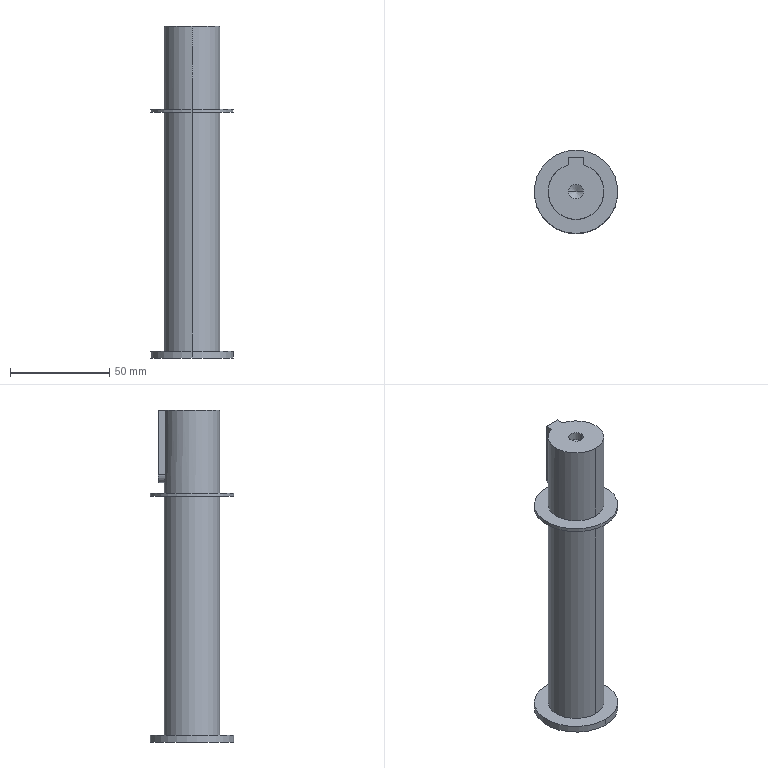Part | SolidWorks | features ICE 3, BaseBody 1 | 1 solid | 22 faces | box 42 x 42 x 167 mm | volume 107574 mm3 | cylinder 12 | plane 8 | cone 2 | commonest cylinder face diameters 28 x4 42 x4 7.35 x2 8 x2
STEP:
#1=CARTESIAN_POINT('',(-3.675,0.,99.328));
#2=VERTEX_POINT('',#1);
#3=CARTESIAN_POINT('',(3.675,0.,99.328));
#4=VERTEX_POINT('',#3);
#5=CARTESIAN_POINT('',(0.,0.,99.328));
#6=DIRECTION('',(0.,0.,1.));
#7=DIRECTION('',(1.,0.,0.));
#8=AXIS2_PLACEMENT_3D('',#5,#6,#7);
#9=CIRCLE('',#8,3.675);
#10=EDGE_CURVE('',#2,#4,#9,.T.);
#11=ORIENTED_EDGE('',*,*,#10,.F.);
#12=CARTESIAN_POINT('',(-3.675,0.,103.5));
#13=VERTEX_POINT('',#12);
#14=CARTESIAN_POINT('',(-3.675,0.,97.206));
#15=DIRECTION('',(0.,0.,1.));
#16=VECTOR('',#15,1000.);
#17=LINE('',#14,#16);
#18=EDGE_CURVE('',#2,#13,#17,.T.);
#19=ORIENTED_EDGE('',*,*,#18,.T.);
#20=CARTESIAN_POINT('',(3.675,0.,103.5));
#21=VERTEX_POINT('',#20);
#22=CARTESIAN_POINT('',(0.,0.,103.5));
#23=DIRECTION('',(0.,0.,-1.));
#24=DIRECTION('',(1.,0.,0.));
#25=AXIS2_PLACEMENT_3D('',#22,#23,#24);
#26=CIRCLE('',#25,3.675);
#27=EDGE_CURVE('',#21,#13,#26,.T.);
#28=ORIENTED_EDGE('',*,*,#27,.F.);
#29=CARTESIAN_POINT('',(3.675,0.,97.206));
#30=DIRECTION('',(0.,0.,1.));
#31=VECTOR('',#30,1000.);
#32=LINE('',#29,#31);
#33=EDGE_CURVE('',#4,#21,#32,.T.);
#34=ORIENTED_EDGE('',*,*,#33,.F.);
#35=EDGE_LOOP('',(#11,#19,#28,#34));
#36=FACE_OUTER_BOUND('',#35,.T.);
#37=CARTESIAN_POINT('',(0.,0.,97.206));
#38=DIRECTION('',(0.,0.,1.));
#39=DIRECTION('',(1.,0.,0.));
#40=AXIS2_PLACEMENT_3D('',#37,#38,#39);
#41=CYLINDRICAL_SURFACE('',#40,3.675);
#42=ADVANCED_FACE('',(#36),#41,.F.);
#43=CARTESIAN_POINT('',(0.,0.,97.206));
#44=VERTEX_POINT('',#43);
#45=CARTESIAN_POINT('',(3.675,0.,99.328));
#46=DIRECTION('',(0.866,0.,0.5));
#47=VECTOR('',#46,1000.);
#48=LINE('',#45,#47);
#49=EDGE_CURVE('',#44,#4,#48,.T.);
#50=ORIENTED_EDGE('',*,*,#49,.F.);
#51=CARTESIAN_POINT('',(-3.675,0.,99.328));
#52=DIRECTION('',(-0.866,0.,0.5));
#53=VECTOR('',#52,1000.);
#54=LINE('',#51,#53);
#55=EDGE_CURVE('',#44,#2,#54,.T.);
#56=ORIENTED_EDGE('',*,*,#55,.T.);
#57=ORIENTED_EDGE('',*,*,#10,.T.);
#58=EDGE_LOOP('',(#50,#56,#57));
#59=FACE_OUTER_BOUND('',#58,.T.);
#60=CARTESIAN_POINT('',(0.,0.,99.328));
#61=DIRECTION('',(0.,0.,1.));
#62=DIRECTION('',(1.,0.,0.));
#63=AXIS2_PLACEMENT_3D('',#60,#61,#62);
#64=CONICAL_SURFACE('',#63,3.675,1.047);
#65=ADVANCED_FACE('',(#59),#64,.F.);
#66=CARTESIAN_POINT('',(0.,-14.,-60.));
#67=VERTEX_POINT('',#66);
#68=CARTESIAN_POINT('',(0.,14.,-60.));
#69=VERTEX_POINT('',#68);
#70=CARTESIAN_POINT('',(0.,0.,-60.));
#71=DIRECTION('',(0.,0.,1.));
#72=DIRECTION('',(0.,-1.,0.));
#73=AXIS2_PLACEMENT_3D('',#70,#71,#72);
#74=CIRCLE('',#73,14.);
#75=EDGE_CURVE('',#67,#69,#74,.T.);
#76=ORIENTED_EDGE('',*,*,#75,.T.);
#77=CARTESIAN_POINT('',(0.,14.,60.));
#78=VERTEX_POINT('',#77);
#79=CARTESIAN_POINT('',(0.,14.,68.5));
#80=DIRECTION('',(0.,0.,1.));
#81=VECTOR('',#80,1000.);
#82=LINE('',#79,#81);
#83=EDGE_CURVE('',#69,#78,#82,.T.);
#84=ORIENTED_EDGE('',*,*,#83,.T.);
#85=CARTESIAN_POINT('',(0.,-14.,60.));
#86=VERTEX_POINT('',#85);
#87=CARTESIAN_POINT('',(0.,0.,60.));
#88=DIRECTION('',(0.,0.,-1.));
#89=DIRECTION('',(0.,-1.,0.));
#90=AXIS2_PLACEMENT_3D('',#87,#88,#89);
#91=CIRCLE('',#90,14.);
#92=EDGE_CURVE('',#78,#86,#91,.T.);
#93=ORIENTED_EDGE('',*,*,#92,.T.);
#94=CARTESIAN_POINT('',(0.,-14.,68.5));
#95=DIRECTION('',(0.,0.,1.));
#96=VECTOR('',#95,1000.);
#97=LINE('',#94,#96);
#98=EDGE_CURVE('',#67,#86,#97,.T.);
#99=ORIENTED_EDGE('',*,*,#98,.F.);
#100=EDGE_LOOP('',(#76,#84,#93,#99));
#101=FACE_OUTER_BOUND('',#100,.T.);
#102=CARTESIAN_POINT('',(0.,0.,68.5));
#103=DIRECTION('',(0.,0.,1.));
#104=DIRECTION('',(0.,-1.,0.));
#105=AXIS2_PLACEMENT_3D('',#102,#103,#104);
#106=CYLINDRICAL_SURFACE('',#105,14.);
#107=ADVANCED_FACE('',(#101),#106,.T.);
#108=CARTESIAN_POINT('',(0.,-21.,60.));
#109=VERTEX_POINT('',#108);
#110=CARTESIAN_POINT('',(0.,21.,60.));
#111=VERTEX_POINT('',#110);
#112=CARTESIAN_POINT('',(0.,0.,60.));
#113=DIRECTION('',(0.,0.,1.));
#114=DIRECTION('',(0.,-1.,0.));
#115=AXIS2_PLACEMENT_3D('',#112,#113,#114);
#116=CIRCLE('',#115,21.);
#117=EDGE_CURVE('',#109,#111,#116,.T.);
#118=ORIENTED_EDGE('',*,*,#117,.T.);
#119=CARTESIAN_POINT('',(0.,21.,61.75));
#120=VERTEX_POINT('',#119);
#121=CARTESIAN_POINT('',(0.,21.,68.5));
#122=DIRECTION('',(0.,0.,1.));
#123=VECTOR('',#122,1000.);
#124=LINE('',#121,#123);
#125=EDGE_CURVE('',#111,#120,#124,.T.);
#126=ORIENTED_EDGE('',*,*,#125,.T.);
#127=CARTESIAN_POINT('',(0.,-21.,61.75));
#128=VERTEX_POINT('',#127);
#129=CARTESIAN_POINT('',(0.,0.,61.75));
#130=DIRECTION('',(0.,0.,-1.));
#131=DIRECTION('',(0.,-1.,0.));
#132=AXIS2_PLACEMENT_3D('',#129,#130,#131);
#133=CIRCLE('',#132,21.);
#134=EDGE_CURVE('',#120,#128,#133,.T.);
#135=ORIENTED_EDGE('',*,*,#134,.T.);
#136=CARTESIAN_POINT('',(0.,-21.,68.5));
#137=DIRECTION('',(0.,0.,1.));
#138=VECTOR('',#137,1000.);
#139=LINE('',#136,#138);
#140=EDGE_CURVE('',#109,#128,#139,.T.);
#141=ORIENTED_EDGE('',*,*,#140,.F.);
#142=EDGE_LOOP('',(#118,#126,#135,#141));
#143=FACE_OUTER_BOUND('',#142,.T.);
#144=CARTESIAN_POINT('',(0.,0.,68.5));
#145=DIRECTION('',(0.,0.,1.));
#146=DIRECTION('',(0.,-1.,0.));
#147=AXIS2_PLACEMENT_3D('',#144,#145,#146);
#148=CYLINDRICAL_SURFACE('',#147,21.);
#149=ADVANCED_FACE('',(#143),#148,.T.);
#150=CARTESIAN_POINT('',(0.,-21.,-63.5));
#151=VERTEX_POINT('',#150);
#152=CARTESIAN_POINT('',(0.,21.,-63.5));
#153=VERTEX_POINT('',#152);
#154=CARTESIAN_POINT('',(0.,0.,-63.5));
#155=DIRECTION('',(0.,0.,1.));
#156=DIRECTION('',(0.,-1.,0.));
#157=AXIS2_PLACEMENT_3D('',#154,#155,#156);
#158=CIRCLE('',#157,21.);
#159=EDGE_CURVE('',#151,#153,#158,.T.);
#160=ORIENTED_EDGE('',*,*,#159,.T.);
#161=CARTESIAN_POINT('',(0.,21.,-60.));
#162=VERTEX_POINT('',#161);
#163=CARTESIAN_POINT('',(0.,21.,68.5));
#164=DIRECTION('',(0.,0.,1.));
#165=VECTOR('',#164,1000.);
#166=LINE('',#163,#165);
#167=EDGE_CURVE('',#153,#162,#166,.T.);
#168=ORIENTED_EDGE('',*,*,#167,.T.);
#169=CARTESIAN_POINT('',(0.,-21.,-60.));
#170=VERTEX_POINT('',#169);
#171=CARTESIAN_POINT('',(0.,0.,-60.));
#172=DIRECTION('',(0.,0.,-1.));
#173=DIRECTION('',(0.,-1.,0.));
#174=AXIS2_PLACEMENT_3D('',#171,#172,#173);
#175=CIRCLE('',#174,21.);
#176=EDGE_CURVE('',#162,#170,#175,.T.);
#177=ORIENTED_EDGE('',*,*,#176,.T.);
#178=CARTESIAN_POINT('',(0.,-21.,68.5));
#179=DIRECTION('',(0.,0.,1.));
#180=VECTOR('',#179,1000.);
#181=LINE('',#178,#180);
#182=EDGE_CURVE('',#151,#170,#181,.T.);
#183=ORIENTED_EDGE('',*,*,#182,.F.);
#184=EDGE_LOOP('',(#160,#168,#177,#183));
#185=FACE_OUTER_BOUND('',#184,.T.);
#186=CARTESIAN_POINT('',(0.,0.,68.5));
#187=DIRECTION('',(0.,0.,1.));
#188=DIRECTION('',(0.,-1.,0.));
#189=AXIS2_PLACEMENT_3D('',#186,#187,#188);
#190=CYLINDRICAL_SURFACE('',#189,21.);
#191=ADVANCED_FACE('',(#185),#190,.T.);
#192=CARTESIAN_POINT('',(-4.,17.,71.));
#193=VERTEX_POINT('',#192);
#194=CARTESIAN_POINT('',(0.,17.,67.));
#195=VERTEX_POINT('',#194);
#196=CARTESIAN_POINT('',(0.,17.,71.));
#197=DIRECTION('',(0.,-1.,0.));
#198=DIRECTION('',(0.,0.,-1.));
#199=AXIS2_PLACEMENT_3D('',#196,#197,#198);
#200=CIRCLE('',#199,4.);
#201=EDGE_CURVE('',#193,#195,#200,.T.);
#202=ORIENTED_EDGE('',*,*,#201,.T.);
#203=CARTESIAN_POINT('',(0.,14.,67.));
#204=VERTEX_POINT('',#203);
#205=CARTESIAN_POINT('',(0.,17.,67.));
#206=DIRECTION('',(0.,-1.,0.));
#207=VECTOR('',#206,1000.);
#208=LINE('',#205,#207);
#209=EDGE_CURVE('',#195,#204,#208,.T.);
#210=ORIENTED_EDGE('',*,*,#209,.T.);
#211=CARTESIAN_POINT('',(-4.,13.416,71.));
#212=VERTEX_POINT('',#211);
#213=CARTESIAN_POINT('',(-4.,13.416,71.));
#214=CARTESIAN_POINT('',(-4.,13.416,70.734));
#215=CARTESIAN_POINT('',(-3.974,13.424,70.474));
#216=CARTESIAN_POINT('',(-3.871,13.454,69.961));
#217=CARTESIAN_POINT('',(-3.794,13.477,69.706));
#218=CARTESIAN_POINT('',(-3.593,13.531,69.223));
#219=CARTESIAN_POINT('',(-3.47,13.564,68.994));
#220=CARTESIAN_POINT('',(-3.18,13.635,68.56));
#221=CARTESIAN_POINT('',(-3.013,13.673,68.356));
#222=CARTESIAN_POINT('',(-2.646,13.749,67.989));
#223=CARTESIAN_POINT('',(-2.446,13.786,67.824));
#224=CARTESIAN_POINT('',(-2.009,13.857,67.531));
#225=CARTESIAN_POINT('',(-1.779,13.889,67.408));
#226=CARTESIAN_POINT('',(-1.299,13.942,67.208));
#227=CARTESIAN_POINT('',(-1.046,13.963,67.13));
#228=CARTESIAN_POINT('',(-0.5278,13.992,67.026));
#229=CARTESIAN_POINT('',(-0.2656,14.,67.));
#230=CARTESIAN_POINT('',(0.,14.,67.));
#231=B_SPLINE_CURVE_WITH_KNOTS('',3,(#213,#214,#215,#216,#217,#218,#219,#220,#221,#222,#223,#224,#225,#226,#227,#228,#229,#230),.UNSPECIFIED.,.F.,.F.,(4,2,2,2,2,2,2,2,4),(-0.006282,-0.005496,-0.004711,-0.003926,-0.003141,-0.002356,-0.00157,-0.0007852,0.),.UNSPECIFIED.);
#232=EDGE_CURVE('',#212,#204,#231,.T.);
#233=ORIENTED_EDGE('',*,*,#232,.F.);
#234=CARTESIAN_POINT('',(-4.,17.,71.));
#235=DIRECTION('',(0.,1.,0.));
#236=VECTOR('',#235,1000.);
#237=LINE('',#234,#236);
#238=EDGE_CURVE('',#212,#193,#237,.T.);
#239=ORIENTED_EDGE('',*,*,#238,.T.);
#240=EDGE_LOOP('',(#202,#210,#233,#239));
#241=FACE_OUTER_BOUND('',#240,.T.);
#242=CARTESIAN_POINT('',(0.,17.,71.));
#243=DIRECTION('',(0.,-1.,0.));
#244=DIRECTION('',(0.,0.,-1.));
#245=AXIS2_PLACEMENT_3D('',#242,#243,#244);
#246=CYLINDRICAL_SURFACE('',#245,4.);
#247=ADVANCED_FACE('',(#241),#246,.T.);
#248=CARTESIAN_POINT('',(0.,-14.,61.75));
#249=VERTEX_POINT('',#248);
#250=CARTESIAN_POINT('',(0.,14.,61.75));
#251=VERTEX_POINT('',#250);
#252=CARTESIAN_POINT('',(0.,0.,61.75));
#253=DIRECTION('',(0.,0.,1.));
#254=DIRECTION('',(0.,-1.,0.));
#255=AXIS2_PLACEMENT_3D('',#252,#253,#254);
#256=CIRCLE('',#255,14.);
#257=EDGE_CURVE('',#249,#251,#256,.T.);
#258=ORIENTED_EDGE('',*,*,#257,.T.);
#259=CARTESIAN_POINT('',(0.,14.,68.5));
#260=DIRECTION('',(0.,0.,1.));
#261=VECTOR('',#260,1000.);
#262=LINE('',#259,#261);
#263=EDGE_CURVE('',#251,#204,#262,.T.);
#264=ORIENTED_EDGE('',*,*,#263,.T.);
#265=CARTESIAN_POINT('',(4.,13.416,71.));
#266=VERTEX_POINT('',#265);
#267=CARTESIAN_POINT('',(0.,14.,67.));
#268=CARTESIAN_POINT('',(0.2656,14.,67.));
#269=CARTESIAN_POINT('',(0.5265,13.992,67.026));
#270=CARTESIAN_POINT('',(1.039,13.964,67.129));
#271=CARTESIAN_POINT('',(1.294,13.942,67.206));
#272=CARTESIAN_POINT('',(1.778,13.889,67.407));
#273=CARTESIAN_POINT('',(2.007,13.857,67.53));
#274=CARTESIAN_POINT('',(2.44,13.787,67.82));
#275=CARTESIAN_POINT('',(2.645,13.749,67.988));
#276=CARTESIAN_POINT('',(3.011,13.674,68.354));
#277=CARTESIAN_POINT('',(3.176,13.636,68.555));
#278=CARTESIAN_POINT('',(3.469,13.564,68.991));
#279=CARTESIAN_POINT('',(3.592,13.532,69.221));
#280=CARTESIAN_POINT('',(3.792,13.477,69.702));
#281=CARTESIAN_POINT('',(3.87,13.455,69.954));
#282=CARTESIAN_POINT('',(3.974,13.424,70.472));
#283=CARTESIAN_POINT('',(4.,13.416,70.734));
#284=CARTESIAN_POINT('',(4.,13.416,71.));
#285=B_SPLINE_CURVE_WITH_KNOTS('',3,(#267,#268,#269,#270,#271,#272,#273,#274,#275,#276,#277,#278,#279,#280,#281,#282,#283,#284),.UNSPECIFIED.,.F.,.F.,(4,2,2,2,2,2,2,2,4),(0.,0.0007852,0.00157,0.002356,0.003141,0.003926,0.004711,0.005496,0.006282),.UNSPECIFIED.);
#286=EDGE_CURVE('',#204,#266,#285,.T.);
#287=ORIENTED_EDGE('',*,*,#286,.T.);
#288=CARTESIAN_POINT('',(4.,13.416,103.5));
#289=VERTEX_POINT('',#288);
#290=CARTESIAN_POINT('',(4.,13.416,68.5));
#291=DIRECTION('',(0.,0.,1.));
#292=VECTOR('',#291,1000.);
#293=LINE('',#290,#292);
#294=EDGE_CURVE('',#266,#289,#293,.T.);
#295=ORIENTED_EDGE('',*,*,#294,.T.);
#296=CARTESIAN_POINT('',(0.,-14.,103.5));
#297=VERTEX_POINT('',#296);
#298=CARTESIAN_POINT('',(0.,0.,103.5));
#299=DIRECTION('',(0.,0.,-1.));
#300=DIRECTION('',(1.,0.,0.));
#301=AXIS2_PLACEMENT_3D('',#298,#299,#300);
#302=CIRCLE('',#301,14.);
#303=EDGE_CURVE('',#289,#297,#302,.T.);
#304=ORIENTED_EDGE('',*,*,#303,.T.);
#305=CARTESIAN_POINT('',(0.,-14.,68.5));
#306=DIRECTION('',(0.,0.,1.));
#307=VECTOR('',#306,1000.);
#308=LINE('',#305,#307);
#309=EDGE_CURVE('',#249,#297,#308,.T.);
#310=ORIENTED_EDGE('',*,*,#309,.F.);
#311=EDGE_LOOP('',(#258,#264,#287,#295,#304,#310));
#312=FACE_OUTER_BOUND('',#311,.T.);
#313=CARTESIAN_POINT('',(0.,0.,68.5));
#314=DIRECTION('',(0.,0.,1.));
#315=DIRECTION('',(0.,-1.,0.));
#316=AXIS2_PLACEMENT_3D('',#313,#314,#315);
#317=CYLINDRICAL_SURFACE('',#316,14.);
#318=ADVANCED_FACE('',(#312),#317,.T.);
#319=CARTESIAN_POINT('',(4.,17.,103.5));
#320=VERTEX_POINT('',#319);
#321=CARTESIAN_POINT('',(-4.,17.,103.5));
#322=VERTEX_POINT('',#321);
#323=CARTESIAN_POINT('',(0.,17.,103.5));
#324=DIRECTION('',(-1.,0.,0.));
#325=VECTOR('',#324,1000.);
#326=LINE('',#323,#325);
#327=EDGE_CURVE('',#320,#322,#326,.T.);
#328=ORIENTED_EDGE('',*,*,#327,.F.);
#329=CARTESIAN_POINT('',(4.,17.,71.));
#330=VERTEX_POINT('',#329);
#331=CARTESIAN_POINT('',(4.,17.,71.));
#332=DIRECTION('',(0.,0.,-1.));
#333=VECTOR('',#332,1000.);
#334=LINE('',#331,#333);
#335=EDGE_CURVE('',#320,#330,#334,.T.);
#336=ORIENTED_EDGE('',*,*,#335,.T.);
#337=CARTESIAN_POINT('',(0.,17.,71.));
#338=DIRECTION('',(0.,-1.,0.));
#339=DIRECTION('',(0.,0.,-1.));
#340=AXIS2_PLACEMENT_3D('',#337,#338,#339);
#341=CIRCLE('',#340,4.);
#342=EDGE_CURVE('',#195,#330,#341,.T.);
#343=ORIENTED_EDGE('',*,*,#342,.F.);
#344=ORIENTED_EDGE('',*,*,#201,.F.);
#345=CARTESIAN_POINT('',(-4.,17.,115.3));
#346=DIRECTION('',(0.,0.,1.));
#347=VECTOR('',#346,1000.);
#348=LINE('',#345,#347);
#349=EDGE_CURVE('',#193,#322,#348,.T.);
#350=ORIENTED_EDGE('',*,*,#349,.T.);
#351=EDGE_LOOP('',(#328,#336,#343,#344,#350));
#352=FACE_OUTER_BOUND('',#351,.T.);
#353=CARTESIAN_POINT('',(0.,17.,115.3));
#354=DIRECTION('',(0.,-1.,0.));
#355=DIRECTION('',(0.,0.,-1.));
#356=AXIS2_PLACEMENT_3D('',#353,#354,#355);
#357=PLANE('',#356);
#358=ADVANCED_FACE('',(#352),#357,.F.);
#359=CARTESIAN_POINT('',(-4.,13.416,103.5));
#360=VERTEX_POINT('',#359);
#361=CARTESIAN_POINT('',(-4.,17.,103.5));
#362=DIRECTION('',(0.,-1.,0.));
#363=VECTOR('',#362,1000.);
#364=LINE('',#361,#363);
#365=EDGE_CURVE('',#322,#360,#364,.T.);
#366=ORIENTED_EDGE('',*,*,#365,.F.);
#367=ORIENTED_EDGE('',*,*,#349,.F.);
#368=ORIENTED_EDGE('',*,*,#238,.F.);
#369=CARTESIAN_POINT('',(-4.,13.416,68.5));
#370=DIRECTION('',(0.,0.,-1.));
#371=VECTOR('',#370,1000.);
#372=LINE('',#369,#371);
#373=EDGE_CURVE('',#360,#212,#372,.T.);
#374=ORIENTED_EDGE('',*,*,#373,.F.);
#375=EDGE_LOOP('',(#366,#367,#368,#374));
#376=FACE_OUTER_BOUND('',#375,.T.);
#377=CARTESIAN_POINT('',(-4.,17.,115.3));
#378=DIRECTION('',(1.,0.,0.));
#379=DIRECTION('',(0.,0.,-1.));
#380=AXIS2_PLACEMENT_3D('',#377,#378,#379);
#381=PLANE('',#380);
#382=ADVANCED_FACE('',(#376),#381,.F.);
#383=CARTESIAN_POINT('',(4.,17.,103.5));
#384=DIRECTION('',(0.,1.,0.));
#385=VECTOR('',#384,1000.);
#386=LINE('',#383,#385);
#387=EDGE_CURVE('',#289,#320,#386,.T.);
#388=ORIENTED_EDGE('',*,*,#387,.F.);
#389=ORIENTED_EDGE('',*,*,#294,.F.);
#390=CARTESIAN_POINT('',(4.,17.,71.));
#391=DIRECTION('',(0.,-1.,0.));
#392=VECTOR('',#391,1000.);
#393=LINE('',#390,#392);
#394=EDGE_CURVE('',#330,#266,#393,.T.);
#395=ORIENTED_EDGE('',*,*,#394,.F.);
#396=ORIENTED_EDGE('',*,*,#335,.F.);
#397=EDGE_LOOP('',(#388,#389,#395,#396));
#398=FACE_OUTER_BOUND('',#397,.T.);
#399=CARTESIAN_POINT('',(4.,17.,71.));
#400=DIRECTION('',(-1.,0.,0.));
#401=DIRECTION('',(0.,0.,1.));
#402=AXIS2_PLACEMENT_3D('',#399,#400,#401);
#403=PLANE('',#402);
#404=ADVANCED_FACE('',(#398),#403,.F.);
#405=ORIENTED_EDGE('',*,*,#263,.F.);
#406=CARTESIAN_POINT('',(0.,0.,61.75));
#407=DIRECTION('',(0.,0.,1.));
#408=DIRECTION('',(0.,-1.,0.));
#409=AXIS2_PLACEMENT_3D('',#406,#407,#408);
#410=CIRCLE('',#409,14.);
#411=EDGE_CURVE('',#251,#249,#410,.T.);
#412=ORIENTED_EDGE('',*,*,#411,.T.);
#413=ORIENTED_EDGE('',*,*,#309,.T.);
#414=CARTESIAN_POINT('',(0.,0.,103.5));
#415=DIRECTION('',(0.,0.,-1.));
#416=DIRECTION('',(1.,0.,0.));
#417=AXIS2_PLACEMENT_3D('',#414,#415,#416);
#418=CIRCLE('',#417,14.);
#419=EDGE_CURVE('',#297,#360,#418,.T.);
#420=ORIENTED_EDGE('',*,*,#419,.T.);
#421=ORIENTED_EDGE('',*,*,#373,.T.);
#422=ORIENTED_EDGE('',*,*,#232,.T.);
#423=EDGE_LOOP('',(#405,#412,#413,#420,#421,#422));
#424=FACE_OUTER_BOUND('',#423,.T.);
#425=CARTESIAN_POINT('',(0.,0.,68.5));
#426=DIRECTION('',(0.,0.,1.));
#427=DIRECTION('',(0.,-1.,0.));
#428=AXIS2_PLACEMENT_3D('',#425,#426,#427);
#429=CYLINDRICAL_SURFACE('',#428,14.);
#430=ADVANCED_FACE('',(#424),#429,.T.);
#431=ORIENTED_EDGE('',*,*,#83,.F.);
#432=CARTESIAN_POINT('',(0.,0.,-60.));
#433=DIRECTION('',(0.,0.,1.));
#434=DIRECTION('',(0.,-1.,0.));
#435=AXIS2_PLACEMENT_3D('',#432,#433,#434);
#436=CIRCLE('',#435,14.);
#437=EDGE_CURVE('',#69,#67,#436,.T.);
#438=ORIENTED_EDGE('',*,*,#437,.T.);
#439=ORIENTED_EDGE('',*,*,#98,.T.);
#440=CARTESIAN_POINT('',(0.,0.,60.));
#441=DIRECTION('',(0.,0.,-1.));
#442=DIRECTION('',(0.,-1.,0.));
#443=AXIS2_PLACEMENT_3D('',#440,#441,#442);
#444=CIRCLE('',#443,14.);
#445=EDGE_CURVE('',#86,#78,#444,.T.);
#446=ORIENTED_EDGE('',*,*,#445,.T.);
#447=EDGE_LOOP('',(#431,#438,#439,#446));
#448=FACE_OUTER_BOUND('',#447,.T.);
#449=CARTESIAN_POINT('',(0.,0.,68.5));
#450=DIRECTION('',(0.,0.,1.));
#451=DIRECTION('',(0.,-1.,0.));
#452=AXIS2_PLACEMENT_3D('',#449,#450,#451);
#453=CYLINDRICAL_SURFACE('',#452,14.);
#454=ADVANCED_FACE('',(#448),#453,.T.);
#455=ORIENTED_EDGE('',*,*,#445,.F.);
#456=ORIENTED_EDGE('',*,*,#92,.F.);
#457=EDGE_LOOP('',(#455,#456));
#458=FACE_BOUND('',#457,.T.);
#459=ORIENTED_EDGE('',*,*,#117,.F.);
#460=CARTESIAN_POINT('',(0.,0.,60.));
#461=DIRECTION('',(0.,0.,1.));
#462=DIRECTION('',(0.,-1.,0.));
#463=AXIS2_PLACEMENT_3D('',#460,#461,#462);
#464=CIRCLE('',#463,21.);
#465=EDGE_CURVE('',#111,#109,#464,.T.);
#466=ORIENTED_EDGE('',*,*,#465,.F.);
#467=EDGE_LOOP('',(#459,#466));
#468=FACE_OUTER_BOUND('',#467,.T.);
#469=CARTESIAN_POINT('',(0.,21.,60.));
#470=DIRECTION('',(0.,0.,1.));
#471=DIRECTION('',(0.,-1.,0.));
#472=AXIS2_PLACEMENT_3D('',#469,#470,#471);
#473=PLANE('',#472);
#474=ADVANCED_FACE('',(#458,#468),#473,.F.);
#475=CARTESIAN_POINT('',(0.,0.,-60.));
#476=DIRECTION('',(0.,0.,-1.));
#477=DIRECTION('',(0.,-1.,0.));
#478=AXIS2_PLACEMENT_3D('',#475,#476,#477);
#479=CIRCLE('',#478,21.);
#480=EDGE_CURVE('',#170,#162,#479,.T.);
#481=ORIENTED_EDGE('',*,*,#480,.F.);
#482=ORIENTED_EDGE('',*,*,#176,.F.);
#483=EDGE_LOOP('',(#481,#482));
#484=FACE_OUTER_BOUND('',#483,.T.);
#485=ORIENTED_EDGE('',*,*,#75,.F.);
#486=ORIENTED_EDGE('',*,*,#437,.F.);
#487=EDGE_LOOP('',(#485,#486));
#488=FACE_BOUND('',#487,.T.);
#489=CARTESIAN_POINT('',(0.,21.,-60.));
#490=DIRECTION('',(0.,0.,-1.));
#491=DIRECTION('',(0.,1.,0.));
#492=AXIS2_PLACEMENT_3D('',#489,#490,#491);
#493=PLANE('',#492);
#494=ADVANCED_FACE('',(#484,#488),#493,.F.);
#495=ORIENTED_EDGE('',*,*,#125,.F.);
#496=ORIENTED_EDGE('',*,*,#465,.T.);
#497=ORIENTED_EDGE('',*,*,#140,.T.);
#498=CARTESIAN_POINT('',(0.,0.,61.75));
#499=DIRECTION('',(0.,0.,-1.));
#500=DIRECTION('',(0.,-1.,0.));
#501=AXIS2_PLACEMENT_3D('',#498,#499,#500);
#502=CIRCLE('',#501,21.);
#503=EDGE_CURVE('',#128,#120,#502,.T.);
#504=ORIENTED_EDGE('',*,*,#503,.T.);
#505=EDGE_LOOP('',(#495,#496,#497,#504));
#506=FACE_OUTER_BOUND('',#505,.T.);
#507=CARTESIAN_POINT('',(0.,0.,68.5));
#508=DIRECTION('',(0.,0.,1.));
#509=DIRECTION('',(0.,-1.,0.));
#510=AXIS2_PLACEMENT_3D('',#507,#508,#509);
#511=CYLINDRICAL_SURFACE('',#510,21.);
#512=ADVANCED_FACE('',(#506),#511,.T.);
#513=ORIENTED_EDGE('',*,*,#167,.F.);
#514=CARTESIAN_POINT('',(0.,0.,-63.5));
#515=DIRECTION('',(0.,0.,1.));
#516=DIRECTION('',(0.,-1.,0.));
#517=AXIS2_PLACEMENT_3D('',#514,#515,#516);
#518=CIRCLE('',#517,21.);
#519=EDGE_CURVE('',#153,#151,#518,.T.);
#520=ORIENTED_EDGE('',*,*,#519,.T.);
#521=ORIENTED_EDGE('',*,*,#182,.T.);
#522=ORIENTED_EDGE('',*,*,#480,.T.);
#523=EDGE_LOOP('',(#513,#520,#521,#522));
#524=FACE_OUTER_BOUND('',#523,.T.);
#525=CARTESIAN_POINT('',(0.,0.,68.5));
#526=DIRECTION('',(0.,0.,1.));
#527=DIRECTION('',(0.,-1.,0.));
#528=AXIS2_PLACEMENT_3D('',#525,#526,#527);
#529=CYLINDRICAL_SURFACE('',#528,21.);
#530=ADVANCED_FACE('',(#524),#529,.T.);
#531=ORIENTED_EDGE('',*,*,#503,.F.);
#532=ORIENTED_EDGE('',*,*,#134,.F.);
#533=EDGE_LOOP('',(#531,#532));
#534=FACE_OUTER_BOUND('',#533,.T.);
#535=ORIENTED_EDGE('',*,*,#257,.F.);
#536=ORIENTED_EDGE('',*,*,#411,.F.);
#537=EDGE_LOOP('',(#535,#536));
#538=FACE_BOUND('',#537,.T.);
#539=CARTESIAN_POINT('',(0.,14.,61.75));
#540=DIRECTION('',(0.,0.,-1.));
#541=DIRECTION('',(0.,1.,0.));
#542=AXIS2_PLACEMENT_3D('',#539,#540,#541);
#543=PLANE('',#542);
#544=ADVANCED_FACE('',(#534,#538),#543,.F.);
#545=ORIENTED_EDGE('',*,*,#159,.F.);
#546=ORIENTED_EDGE('',*,*,#519,.F.);
#547=EDGE_LOOP('',(#545,#546));
#548=FACE_OUTER_BOUND('',#547,.T.);
#549=CARTESIAN_POINT('',(0.,14.,-63.5));
#550=DIRECTION('',(0.,0.,1.));
#551=DIRECTION('',(0.,-1.,0.));
#552=AXIS2_PLACEMENT_3D('',#549,#550,#551);
#553=PLANE('',#552);
#554=ADVANCED_FACE('',(#548),#553,.F.);
#555=ORIENTED_EDGE('',*,*,#209,.F.);
#556=ORIENTED_EDGE('',*,*,#342,.T.);
#557=ORIENTED_EDGE('',*,*,#394,.T.);
#558=ORIENTED_EDGE('',*,*,#286,.F.);
#559=EDGE_LOOP('',(#555,#556,#557,#558));
#560=FACE_OUTER_BOUND('',#559,.T.);
#561=CARTESIAN_POINT('',(0.,17.,71.));
#562=DIRECTION('',(0.,-1.,0.));
#563=DIRECTION('',(0.,0.,-1.));
#564=AXIS2_PLACEMENT_3D('',#561,#562,#563);
#565=CYLINDRICAL_SURFACE('',#564,4.);
#566=ADVANCED_FACE('',(#560),#565,.T.);
#567=ORIENTED_EDGE('',*,*,#27,.T.);
#568=CARTESIAN_POINT('',(0.,0.,103.5));
#569=DIRECTION('',(0.,0.,-1.));
#570=DIRECTION('',(1.,0.,0.));
#571=AXIS2_PLACEMENT_3D('',#568,#569,#570);
#572=CIRCLE('',#571,3.675);
#573=EDGE_CURVE('',#13,#21,#572,.T.);
#574=ORIENTED_EDGE('',*,*,#573,.T.);
#575=EDGE_LOOP('',(#567,#574));
#576=FACE_BOUND('',#575,.T.);
#577=ORIENTED_EDGE('',*,*,#327,.T.);
#578=ORIENTED_EDGE('',*,*,#365,.T.);
#579=ORIENTED_EDGE('',*,*,#419,.F.);
#580=ORIENTED_EDGE('',*,*,#303,.F.);
#581=ORIENTED_EDGE('',*,*,#387,.T.);
#582=EDGE_LOOP('',(#577,#578,#579,#580,#581));
#583=FACE_OUTER_BOUND('',#582,.T.);
#584=CARTESIAN_POINT('',(0.,0.,103.5));
#585=DIRECTION('',(0.,0.,1.));
#586=DIRECTION('',(1.,0.,0.));
#587=AXIS2_PLACEMENT_3D('',#584,#585,#586);
#588=PLANE('',#587);
#589=ADVANCED_FACE('',(#576,#583),#588,.T.);
#590=ORIENTED_EDGE('',*,*,#55,.F.);
#591=ORIENTED_EDGE('',*,*,#49,.T.);
#592=CARTESIAN_POINT('',(0.,0.,99.328));
#593=DIRECTION('',(0.,0.,1.));
#594=DIRECTION('',(1.,0.,0.));
#595=AXIS2_PLACEMENT_3D('',#592,#593,#594);
#596=CIRCLE('',#595,3.675);
#597=EDGE_CURVE('',#4,#2,#596,.T.);
#598=ORIENTED_EDGE('',*,*,#597,.T.);
#599=EDGE_LOOP('',(#590,#591,#598));
#600=FACE_OUTER_BOUND('',#599,.T.);
#601=CARTESIAN_POINT('',(0.,0.,99.328));
#602=DIRECTION('',(0.,0.,1.));
#603=DIRECTION('',(1.,0.,0.));
#604=AXIS2_PLACEMENT_3D('',#601,#602,#603);
#605=CONICAL_SURFACE('',#604,3.675,1.047);
#606=ADVANCED_FACE('',(#600),#605,.F.);
#607=ORIENTED_EDGE('',*,*,#18,.F.);
#608=ORIENTED_EDGE('',*,*,#597,.F.);
#609=ORIENTED_EDGE('',*,*,#33,.T.);
#610=ORIENTED_EDGE('',*,*,#573,.F.);
#611=EDGE_LOOP('',(#607,#608,#609,#610));
#612=FACE_OUTER_BOUND('',#611,.T.);
#613=CARTESIAN_POINT('',(0.,0.,97.206));
#614=DIRECTION('',(0.,0.,1.));
#615=DIRECTION('',(1.,0.,0.));
#616=AXIS2_PLACEMENT_3D('',#613,#614,#615);
#617=CYLINDRICAL_SURFACE('',#616,3.675);
#618=ADVANCED_FACE('',(#612),#617,.F.);
#619=CLOSED_SHELL('',(#42,#65,#107,#149,#191,#247,#318,#358,#382,#404,#430,#454,#474,#494,#512,#530,#544,#554,#566,#589,#606,#618));
#620=MANIFOLD_SOLID_BREP('',#619);
#621=CARTESIAN_POINT('',(0.,0.,0.));
#622=DIRECTION('',(0.,0.,1.));
#623=DIRECTION('',(1.,0.,0.));
#624=AXIS2_PLACEMENT_3D('',#621,#622,#623);
#625=(LENGTH_UNIT()NAMED_UNIT(*)SI_UNIT(.MILLI.,.METRE.));
#626=UNCERTAINTY_MEASURE_WITH_UNIT(LENGTH_MEASURE(0.00001),#625,'','');
#627=(NAMED_UNIT(*)PLANE_ANGLE_UNIT()SI_UNIT($,.RADIAN.));
#628=(NAMED_UNIT(*)SI_UNIT($,.STERADIAN.)SOLID_ANGLE_UNIT());
#629=(GEOMETRIC_REPRESENTATION_CONTEXT(3)GLOBAL_UNCERTAINTY_ASSIGNED_CONTEXT((#626))GLOBAL_UNIT_ASSIGNED_CONTEXT((#625,#627,#628))REPRESENTATION_CONTEXT('',''));
#630=ADVANCED_BREP_SHAPE_REPRESENTATION('',(#620,#624),#629);